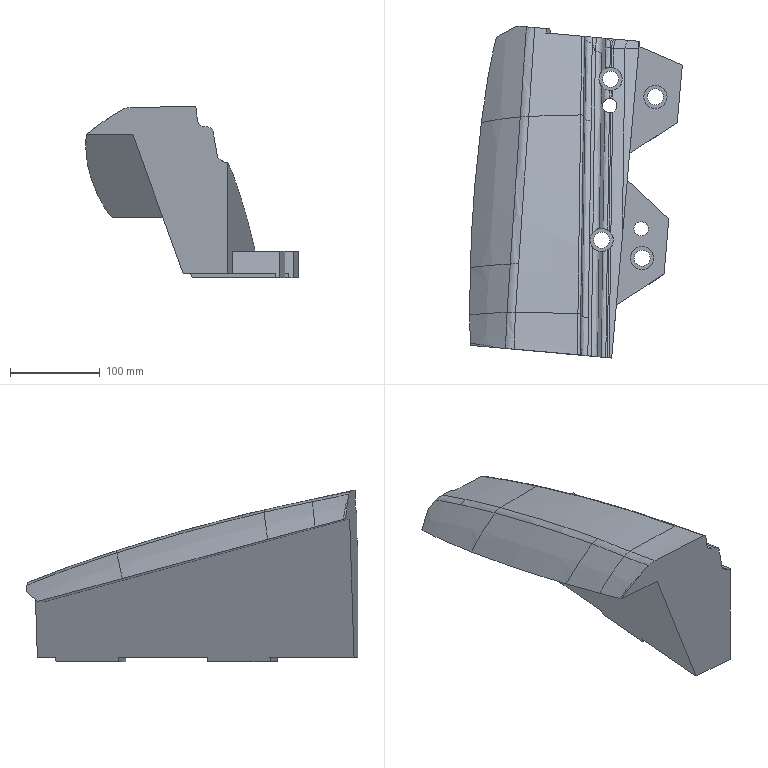Part | NX | features solid 2 | 1 solid | 92 faces | box 237.398 x 370.639 x 191.883 mm | volume 3891162 mm3 | spline 53 | plane 29 | cylinder 10 | commonest cylinder face diameters 18 x4 26 x4 16 x2